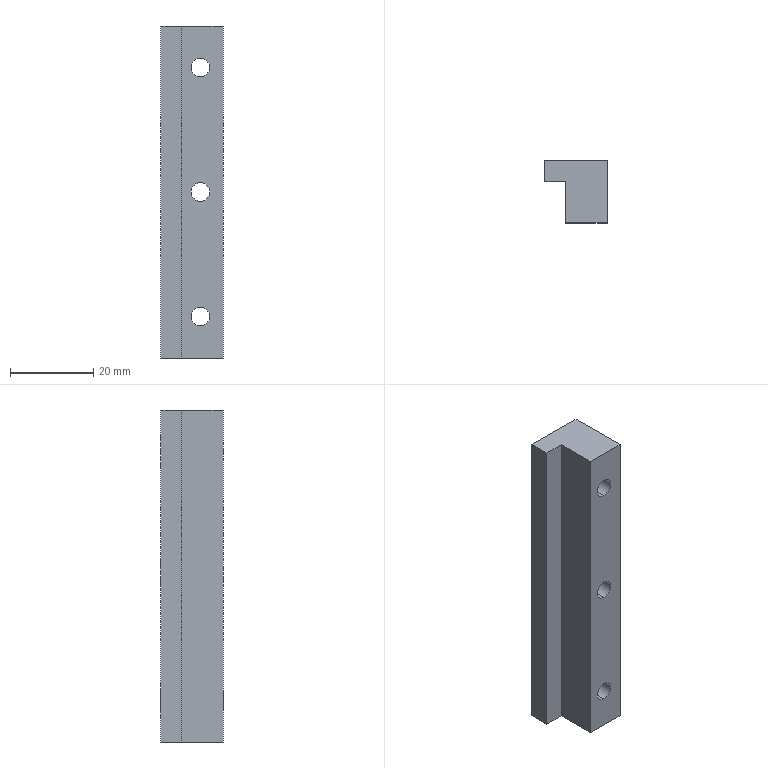Part | STEP file | Guide block | 1 solid | 23 faces | box 15 x 15 x 80 mm | volume 12810 mm3 | cylinder 12 | plane 11 | commonest cylinder face diameters 4.5 x6 8 x6